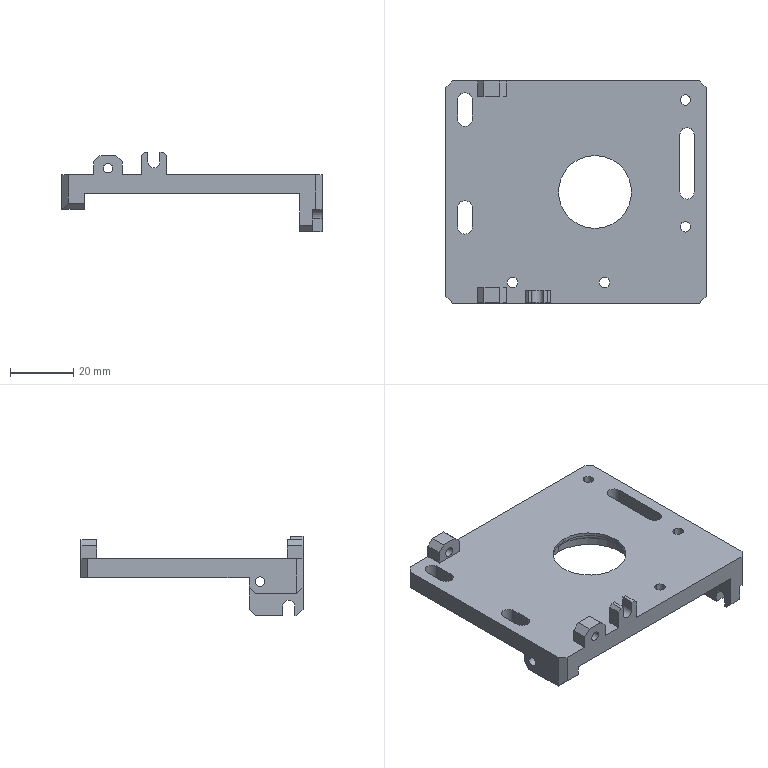NC program | NX | posted with a generic post | part box 82 x 70 x 25 mm
Lines 5584 to 7083 of 7981:
(CAVITY_MILL_COPY , TOOL : D4)
N11148 T04 M6
N11150 G54
N11152 G17 G0 G90 X-14.17 Y-28.2 S9500 M3
N11154 G43 Z30. H4
N11156 Z0.25
N11158 G94 G1 Z-0.25 F1800.
N11160 X-14.123 Y-28.364
N11162 G3 X-13.407 Y-29.062 R1.
N11164 G2 X-12. Y-30.376 R2.
N11166 X-10.593 Y-29.062 R2.
N11168 G3 X-9.877 Y-28.364 R1.
N11170 G1 X-9.83 Y-28.2
N11172 Z0.25
N11174 G0 Z30.
N11176 X-14.17
N11178 Z0.
N11180 G1 Z-0.5
N11182 X-14.123 Y-28.364
N11184 G3 X-13.407 Y-29.062 R1.
N11186 G2 X-12. Y-30.376 R2.
N11188 X-10.593 Y-29.062 R2.
N11190 G3 X-9.877 Y-28.364 R1.
N11192 G1 X-9.83 Y-28.2
N11194 Z0.
N11196 G0 X-14.17 Z-0.25
N11198 G1 Z-0.75
N11200 X-14.123 Y-28.364
N11202 G3 X-13.407 Y-29.062 R1.
N11204 G2 X-12. Y-30.376 R2.
N11206 X-10.593 Y-29.062 R2.
N11208 G3 X-9.877 Y-28.364 R1.
N11210 G1 X-9.83 Y-28.2
N11212 Z-0.25
N11214 G0 X-14.17 Z-0.5
N11216 G1 Z-1.
N11218 X-14.123 Y-28.364
N11220 G3 X-13.407 Y-29.062 R1.
N11222 G2 X-12. Y-30.376 R2.
N11224 X-10.593 Y-29.062 R2.
N11226 G3 X-9.877 Y-28.364 R1.
N11228 G1 X-9.83 Y-28.2
N11230 Z-0.5
N11232 G0 X-21.047 Y-28.181 Z-0.75
N11234 G1 Z-1.25
N11236 X-20.521 Y-29.33
N11238 G3 X-19.706 Y-29.909 R1.
N11240 G1 X-19.875 Y-31.701
N11242 X-19.95 Y-31.693
N11244 Y-33.841
N11246 X-19.8
N11248 Y-31.707
N11250 X-19.875 Y-31.701
N11252 X-19.706 Y-29.909
N11254 X-19.75 Y-29.904
N11256 G2 X-21.552 Y-28.819 R2.52
N11258 G3 X-22.241 Y-28.689 R0.5
N11260 G2 X-21.75 Y-30. R2.002
N11262 G1 Y-35.
N11264 G2 X-22.401 Y-36.474 R2.003
N11266 G3 X-21.712 Y-36.436 R0.5
N11268 G2 X-18.043 Y-36.43 R2.52
N11270 G3 X-17.357 Y-36.469 R0.5
N11272 G2 X-18. Y-35. R2.
N11274 G1 Y-31.
N11276 G2 X-17.172 Y-29.379 R2.
N11278 G3 X-17.857 Y-29.336 R0.5
N11280 G2 X-19.706 Y-29.909 R2.52
N11282 X-20.521 Y-29.33 R1.
N11284 G1 X-21.047 Y-28.181
N11286 Z-0.75
N11288 G0 X-18.039 Y-28.483 Z-1.
N11290 G1 Z-1.5
N11292 X-18.726 Y-29.376
N11294 G2 X-19.65 Y-29.758 R1.
N11296 X-21.319 Y-28.792 R2.52
N11298 G3 X-21.996 Y-28.681 R0.5
N11300 G2 X-21.5 Y-30. R2.
N11302 G1 Y-35.
N11304 G2 X-22.304 Y-36.603 R2.
N11306 G3 X-21.604 Y-36.623 R0.5
N11308 G1 X-21.45 Y-36.48
N11310 G2 X-17.979 Y-36.517 R2.52
N11312 G3 X-17.292 Y-36.527 R0.5
N11314 G2 X-18. Y-35. R2.
N11316 G1 Y-31.
N11318 G2 X-17.104 Y-29.332 R2.
N11320 G3 X-17.787 Y-29.261 R0.5
N11322 G2 X-19.65 Y-29.758 R2.52
N11324 X-20.443 Y-29.148 R1.
N11326 G1 X-20.873 Y-28.106
N11328 Z-1.
N11330 G0 X-17.936 Y-28.402 Z-1.25
N11332 G1 Z-1.75
N11334 X-18.678 Y-29.269
N11336 G2 X-19.621 Y-29.602 R1.
N11338 X-21.111 Y-28.719 R2.52
N11340 G3 X-21.792 Y-28.631 R0.5
N11342 G2 X-21.25 Y-30. R2.
N11344 G1 Y-35.
N11346 G2 X-22. Y-36.562 R2.
N11348 G3 X-21.317 Y-36.574 R0.5
N11350 G2 X-17.929 Y-36.579 R2.52
N11352 G3 X-17.243 Y-36.567 R0.5
N11354 G2 X-18. Y-35. R2.
N11356 G1 Y-31.
N11358 G2 X-17.034 Y-29.288 R2.
N11360 G3 X-17.713 Y-29.188 R0.5
N11362 G2 X-19.621 Y-29.602 R2.52
N11364 X-20.381 Y-28.952 R1.
N11366 G1 X-20.719 Y-27.995
N11368 Z-1.25
N11370 G0 X-17.828 Y-28.324 Z-1.5
N11372 G1 Z-2.
N11374 X-18.624 Y-29.161
N11376 G2 X-19.583 Y-29.445 R1.
N11378 X-20.906 Y-28.635 R2.52
N11380 G1 X-20.927 Y-28.611
N11382 G3 X-21.623 Y-28.55 R0.5
N11384 G2 X-21. Y-30. R2.
N11386 G1 Y-35.
N11388 G2 X-21.822 Y-36.616 R2.
N11390 G3 X-21.133 Y-36.654 R0.5
N11392 G2 X-17.871 Y-36.648 R2.52
N11394 G3 X-17.185 Y-36.611 R0.5
N11396 G2 X-18. Y-35. R2.
N11398 G1 Y-31.
N11400 G2 X-16.96 Y-29.246 R2.
N11402 G3 X-17.635 Y-29.118 R0.5
N11404 G2 X-19.583 Y-29.445 R2.52
N11406 X-20.308 Y-28.756 R1.
N11408 G1 X-20.571 Y-27.864
N11410 Z-1.5
N11412 G0 X-17.729 Y-28.258 Z-1.75
N11414 G1 Z-2.25
N11416 X-18.572 Y-29.066
N11418 G2 X-19.543 Y-29.304 R1.
N11420 X-20.691 Y-28.594 R2.52
N11422 G3 X-21.375 Y-28.547 R0.5
N11424 G2 X-20.75 Y-30. R2.
N11426 G1 Y-35.
N11428 G2 X-21.677 Y-36.688 R2.
N11430 G3 X-20.982 Y-36.762 R0.5
N11432 G1 X-20.928 Y-36.719
N11434 G2 X-17.81 Y-36.715 R2.52
N11436 G3 X-17.126 Y-36.653 R0.5
N11438 G2 X-18. Y-35. R2.
N11440 G1 Y-31.
N11442 G2 X-16.893 Y-29.211 R2.
N11444 G3 X-17.563 Y-29.057 R0.5
N11446 G2 X-19.543 Y-29.304 R2.52
N11448 X-20.235 Y-28.583 R1.
N11450 G1 X-20.428 Y-27.796
N11452 Z-1.75
N11454 G0 X-17.623 Y-28.193 Z-2.
N11456 G1 Z-2.5
N11458 X-18.512 Y-28.969
N11460 G2 X-19.494 Y-29.161 R1.
N11462 X-20.481 Y-28.537 R2.52
N11464 G3 X-21.167 Y-28.509 R0.5
N11466 G2 X-20.5 Y-30. R2.
N11468 G1 Y-35.
N11470 G2 X-21.439 Y-36.695 R2.
N11472 G3 X-20.753 Y-36.78 R0.5
N11474 G2 X-17.754 Y-36.772 R2.52
N11476 G3 X-17.073 Y-36.688 R0.5
N11478 G2 X-18. Y-35. R2.
N11480 G1 Y-31.
N11482 G2 X-16.823 Y-29.177 R2.
N11484 G3 X-17.486 Y-28.998 R0.5
N11486 G2 X-19.494 Y-29.161 R2.52
N11488 X-20.151 Y-28.408 R1.
N11490 G1 X-20.288 Y-27.709
N11492 Z-2.
N11494 G0 X-17.516 Y-28.133 Z-2.25
N11496 G1 Z-2.75
N11498 X-18.449 Y-28.874
N11500 G2 X-19.438 Y-29.021 R1.
N11502 X-20.274 Y-28.479 R2.52
N11504 G3 X-20.962 Y-28.47 R0.5
N11506 G2 X-20.25 Y-30. R2.
N11508 G1 Y-35.
N11510 G2 X-21.231 Y-36.721 R2.
N11512 G3 X-20.553 Y-36.827 R0.5
N11514 G2 X-17.697 Y-36.827 R2.52
N11516 G3 X-17.018 Y-36.721 R0.5
N11518 G2 X-18. Y-35. R2.
N11520 G1 Y-31.
N11522 G2 X-16.752 Y-29.147 R2.
N11524 G3 X-17.407 Y-28.942 R0.5
N11526 G2 X-19.438 Y-29.021 R2.52
N11528 X-20.06 Y-28.237 R1.
N11530 G1 X-20.151 Y-27.626
N11532 Z-2.25
N11534 G0 X-17.41 Y-28.079 Z-2.5
N11536 G1 Z-3.
N11538 X-18.383 Y-28.784
N11540 G2 X-19.378 Y-28.886 R1.
N11542 X-20.062 Y-28.434 R2.52
N11544 G3 X-20.75 Y-28.441 R0.5
N11546 G2 X-20. Y-30.007 R2.009
N11548 G1 Y-34.992
N11550 G2 X-21.039 Y-36.752 R2.004
N11552 G3 X-20.364 Y-36.879 R0.5
N11554 G2 X-17.639 Y-36.879 R2.52
N11556 G3 X-16.964 Y-36.752 R0.5
N11558 G2 X-18. Y-35. R2.
N11560 G1 Y-31.
N11562 G2 X-16.682 Y-29.12 R2.
N11564 G3 X-17.33 Y-28.891 R0.5
N11566 G2 X-19.378 Y-28.886 R2.52
N11568 X-19.964 Y-28.076 R1.
N11570 G1 X-20.018 Y-27.559
N11572 Z-2.5
N11574 G0 X-17.409 Y-28.079 Z-2.75
N11576 G1 Z-3.25
N11578 X-18.383 Y-28.783
N11580 G2 X-19.378 Y-28.885 R1.
N11582 X-20.059 Y-28.435 R2.52
N11584 G3 X-20.745 Y-28.443 R0.5
N11586 G2 X-20. Y-30. R2.
N11588 G1 Y-35.
N11590 G2 X-21.037 Y-36.753 R2.
N11592 G3 X-20.362 Y-36.88 R0.5
N11594 G2 X-17.638 Y-36.88 R2.52
N11596 G3 X-16.963 Y-36.753 R0.5
N11598 G2 X-18. Y-35. R2.
N11600 G1 Y-31.
N11602 G2 X-16.682 Y-29.12 R2.
N11604 G3 X-17.329 Y-28.89 R0.5
N11606 G2 X-19.378 Y-28.885 R2.52
N11608 X-19.964 Y-28.075 R1.
N11610 G1 X-20.017 Y-27.56
N11612 Z-2.75
N11614 G0 X-17.409 Y-28.079 Z-3.
N11616 G1 Z-3.5
N11618 X-18.383 Y-28.783
N11620 G2 X-19.378 Y-28.885 R1.
N11622 X-20.059 Y-28.435 R2.52
N11624 G3 X-20.745 Y-28.443 R0.5
N11626 G2 X-20. Y-30. R2.
N11628 G1 Y-35.
N11630 G2 X-21.037 Y-36.753 R2.
N11632 G3 X-20.362 Y-36.88 R0.5
N11634 G2 X-17.638 Y-36.88 R2.52
N11636 G3 X-16.963 Y-36.753 R0.5
N11638 G2 X-18. Y-35. R2.
N11640 G1 Y-31.
N11642 G2 X-16.682 Y-29.12 R2.
N11644 G3 X-17.329 Y-28.89 R0.5
N11646 G2 X-19.378 Y-28.885 R2.52
N11648 X-19.964 Y-28.075 R1.
N11650 G1 X-20.017 Y-27.56
N11652 Z-3.
N11654 G0 X-17.409 Y-28.079 Z-3.25
N11656 G1 Z-3.75
N11658 X-18.383 Y-28.783
N11660 G2 X-19.378 Y-28.885 R1.
N11662 X-20.059 Y-28.435 R2.52
N11664 G3 X-20.745 Y-28.443 R0.5
N11666 G2 X-20. Y-30. R2.
N11668 G1 Y-35.
N11670 G2 X-21.037 Y-36.753 R2.
N11672 G3 X-20.362 Y-36.88 R0.5
N11674 G2 X-17.638 Y-36.88 R2.52
N11676 G3 X-16.963 Y-36.753 R0.5
N11678 G2 X-18. Y-35. R2.
N11680 G1 Y-31.
N11682 G2 X-16.682 Y-29.12 R2.
N11684 G3 X-17.329 Y-28.89 R0.5
N11686 G2 X-19.378 Y-28.885 R2.52
N11688 X-19.964 Y-28.075 R1.
N11690 G1 X-20.017 Y-27.56
N11692 Z-3.25
N11694 G0 X-17.409 Y-28.079 Z-3.5
N11696 G1 Z-4.
N11698 X-18.383 Y-28.783
N11700 G2 X-19.378 Y-28.885 R1.
N11702 X-20.059 Y-28.435 R2.52
N11704 G3 X-20.745 Y-28.443 R0.5
N11706 G2 X-20. Y-30. R2.
N11708 G1 Y-35.
N11710 G2 X-21.037 Y-36.753 R2.
N11712 G3 X-20.362 Y-36.88 R0.5
N11714 G2 X-17.638 Y-36.88 R2.52
N11716 G3 X-16.963 Y-36.753 R0.5
N11718 G2 X-18. Y-35. R2.
N11720 G1 Y-31.
N11722 G2 X-16.682 Y-29.12 R2.
N11724 G3 X-17.329 Y-28.89 R0.5
N11726 G2 X-19.378 Y-28.885 R2.52
N11728 X-19.964 Y-28.075 R1.
N11730 G1 X-20.017 Y-27.56
N11732 Z-3.5
N11734 G0 X-17.409 Y-28.079 Z-3.75
N11736 G1 Z-4.25
N11738 X-18.383 Y-28.783
N11740 G2 X-19.378 Y-28.885 R1.
N11742 X-20.059 Y-28.435 R2.52
N11744 G3 X-20.745 Y-28.443 R0.5
N11746 G2 X-20. Y-30. R2.
N11748 G1 Y-35.
N11750 G2 X-21.037 Y-36.753 R2.
N11752 G3 X-20.362 Y-36.88 R0.5
N11754 G2 X-17.638 Y-36.88 R2.52
N11756 G3 X-16.963 Y-36.753 R0.5
N11758 G2 X-18. Y-35. R2.
N11760 G1 Y-31.
N11762 G2 X-16.682 Y-29.12 R2.
N11764 G3 X-17.329 Y-28.89 R0.5
N11766 G2 X-19.378 Y-28.885 R2.52
N11768 X-19.964 Y-28.075 R1.
N11770 G1 X-20.017 Y-27.56
N11772 Z-3.75
N11774 G0 X-17.409 Y-28.079 Z-4.
N11776 G1 Z-4.5
N11778 X-18.383 Y-28.783
N11780 G2 X-19.378 Y-28.885 R1.
N11782 X-20.059 Y-28.435 R2.52
N11784 G3 X-20.745 Y-28.443 R0.5
N11786 G2 X-20. Y-30. R2.
N11788 G1 Y-35.
N11790 G2 X-21.037 Y-36.753 R2.
N11792 G3 X-20.362 Y-36.88 R0.5
N11794 G2 X-17.638 Y-36.88 R2.52
N11796 G3 X-16.963 Y-36.753 R0.5
N11798 G2 X-18. Y-35. R2.
N11800 G1 Y-31.
N11802 G2 X-16.682 Y-29.12 R2.
N11804 G3 X-17.329 Y-28.89 R0.5
N11806 G2 X-19.378 Y-28.885 R2.52
N11808 X-19.964 Y-28.075 R1.
N11810 G1 X-20.017 Y-27.56
N11812 Z-4.
N11814 G0 X-17.409 Y-28.079 Z-4.25
N11816 G1 Z-4.75
N11818 X-18.383 Y-28.783
N11820 G2 X-19.378 Y-28.885 R1.
N11822 X-20.059 Y-28.435 R2.52
N11824 G3 X-20.745 Y-28.443 R0.5
N11826 G2 X-20. Y-30. R2.
N11828 G1 Y-35.
N11830 G2 X-21.037 Y-36.753 R2.
N11832 G3 X-20.362 Y-36.88 R0.5
N11834 G2 X-17.638 Y-36.88 R2.52
N11836 G3 X-16.963 Y-36.753 R0.5
N11838 G2 X-18. Y-35. R2.
N11840 G1 Y-31.
N11842 G2 X-16.682 Y-29.12 R2.
N11844 G3 X-17.329 Y-28.89 R0.5
N11846 G2 X-19.378 Y-28.885 R2.52
N11848 X-19.964 Y-28.075 R1.
N11850 G1 X-20.017 Y-27.56
N11852 Z-4.25
N11854 G0 X-17.409 Y-28.079 Z-4.5
N11856 G1 Z-5.
N11858 X-18.383 Y-28.783
N11860 G2 X-19.378 Y-28.885 R1.
N11862 X-20.059 Y-28.435 R2.52
N11864 G3 X-20.745 Y-28.443 R0.5
N11866 G2 X-20. Y-30. R2.
N11868 G1 Y-35.
N11870 G2 X-21.037 Y-36.753 R2.
N11872 G3 X-20.362 Y-36.88 R0.5
N11874 G2 X-17.638 Y-36.88 R2.52
N11876 G3 X-16.963 Y-36.753 R0.5
N11878 G2 X-18. Y-35. R2.
N11880 G1 Y-31.
N11882 G2 X-16.682 Y-29.12 R2.
N11884 G3 X-17.329 Y-28.89 R0.5
N11886 G2 X-19.378 Y-28.885 R2.52
N11888 X-19.964 Y-28.075 R1.
N11890 G1 X-20.017 Y-27.56
N11892 Z-4.5
N11894 G0 X-17.409 Y-28.079 Z-4.75
N11896 G1 Z-5.25
N11898 X-18.383 Y-28.783
N11900 G2 X-19.378 Y-28.885 R1.
N11902 X-20.059 Y-28.435 R2.52
N11904 G3 X-20.745 Y-28.443 R0.5
N11906 G2 X-20. Y-30. R2.
N11908 G1 Y-35.
N11910 G2 X-21.037 Y-36.753 R2.
N11912 G3 X-20.362 Y-36.88 R0.5
N11914 G2 X-17.638 Y-36.88 R2.52
N11916 G3 X-16.963 Y-36.753 R0.5
N11918 G2 X-18. Y-35. R2.
N11920 G1 Y-31.
N11922 G2 X-16.682 Y-29.12 R2.
N11924 G3 X-17.329 Y-28.89 R0.5
N11926 G2 X-19.378 Y-28.885 R2.52
N11928 X-19.964 Y-28.075 R1.
N11930 G1 X-20.017 Y-27.56
N11932 Z-4.75
N11934 G0 X-17.409 Y-28.079 Z-5.
N11936 G1 Z-5.5
N11938 X-18.383 Y-28.783
N11940 G2 X-19.378 Y-28.885 R1.
N11942 X-20.059 Y-28.435 R2.52
N11944 G3 X-20.745 Y-28.443 R0.5
N11946 G2 X-20. Y-30. R2.
N11948 G1 Y-35.
N11950 G2 X-21.037 Y-36.753 R2.
N11952 G3 X-20.362 Y-36.88 R0.5
N11954 G2 X-17.638 Y-36.88 R2.52
N11956 G3 X-16.963 Y-36.753 R0.5
N11958 G2 X-18. Y-35. R2.
N11960 G1 Y-31.
N11962 G2 X-16.682 Y-29.12 R2.
N11964 G3 X-17.329 Y-28.89 R0.5
N11966 G2 X-19.378 Y-28.885 R2.52
N11968 X-19.964 Y-28.075 R1.
N11970 G1 X-20.017 Y-27.56
N11972 Z-5.
N11974 G0 X-17.409 Y-28.079 Z-5.25
N11976 G1 Z-5.75
N11978 X-18.383 Y-28.783
N11980 G2 X-19.378 Y-28.885 R1.
N11982 X-20.059 Y-28.435 R2.52
N11984 G3 X-20.745 Y-28.443 R0.5
N11986 G2 X-20. Y-30. R2.
N11988 G1 Y-35.
N11990 G2 X-21.037 Y-36.753 R2.
N11992 G3 X-20.362 Y-36.88 R0.5
N11994 G2 X-17.638 Y-36.88 R2.52
N11996 G3 X-16.963 Y-36.753 R0.5
N11998 G2 X-18. Y-35. R2.
N12000 G1 Y-31.
N12002 G2 X-16.682 Y-29.12 R2.
N12004 G3 X-17.329 Y-28.89 R0.5
N12006 G2 X-19.378 Y-28.885 R2.52
N12008 X-19.964 Y-28.075 R1.
N12010 G1 X-20.017 Y-27.56
N12012 Z-5.25
N12014 G0 X-17.409 Y-28.079 Z-5.5
N12016 G1 Z-6.
N12018 X-18.383 Y-28.783
N12020 G2 X-19.378 Y-28.885 R1.
N12022 X-20.059 Y-28.435 R2.52
N12024 G3 X-20.745 Y-28.443 R0.5
N12026 G2 X-20. Y-30. R2.
N12028 G1 Y-35.
N12030 G2 X-21.037 Y-36.753 R2.
N12032 G3 X-20.362 Y-36.88 R0.5
N12034 G2 X-17.638 Y-36.88 R2.52
N12036 G3 X-16.963 Y-36.753 R0.5
N12038 G2 X-18. Y-35. R2.
N12040 G1 Y-31.
N12042 G2 X-16.682 Y-29.12 R2.
N12044 G3 X-17.329 Y-28.89 R0.5
N12046 G2 X-19.378 Y-28.885 R2.52
N12048 X-19.964 Y-28.075 R1.
N12050 G1 X-20.017 Y-27.56
N12052 Z-5.5
N12054 G0 X-17.409 Y-28.079 Z-5.75
N12056 G1 Z-6.25
N12058 X-18.383 Y-28.783
N12060 G2 X-19.378 Y-28.885 R1.
N12062 X-20.059 Y-28.435 R2.52
N12064 G3 X-20.745 Y-28.443 R0.5
N12066 G2 X-20. Y-30. R2.
N12068 G1 Y-35.
N12070 G2 X-21.037 Y-36.753 R2.
N12072 G3 X-20.362 Y-36.88 R0.5
N12074 G2 X-17.638 Y-36.88 R2.52
N12076 G3 X-16.963 Y-36.753 R0.5
N12078 G2 X-18. Y-35. R2.
N12080 G1 Y-31.
N12082 G2 X-16.682 Y-29.12 R2.
N12084 G3 X-17.329 Y-28.89 R0.5
N12086 G2 X-19.378 Y-28.885 R2.52
N12088 X-19.964 Y-28.075 R1.
N12090 G1 X-20.017 Y-27.56
N12092 Z-5.75
N12094 G0 X-17.409 Y-28.079 Z-6.
N12096 G1 Z-6.5
N12098 X-18.383 Y-28.783
N12100 G2 X-19.378 Y-28.885 R1.
N12102 X-20.059 Y-28.435 R2.52
N12104 G3 X-20.745 Y-28.443 R0.5
N12106 G2 X-20. Y-30. R2.
N12108 G1 Y-35.
N12110 G2 X-21.037 Y-36.753 R2.
N12112 G3 X-20.362 Y-36.88 R0.5
N12114 G2 X-17.638 Y-36.88 R2.52
N12116 G3 X-16.963 Y-36.753 R0.5
N12118 G2 X-18. Y-35. R2.
N12120 G1 Y-31.
N12122 G2 X-16.682 Y-29.12 R2.
N12124 G3 X-17.329 Y-28.89 R0.5
N12126 G2 X-19.378 Y-28.885 R2.52
N12128 X-19.964 Y-28.075 R1.
N12130 G1 X-20.017 Y-27.56
N12132 Z-6.
N12134 G0 X-17.409 Y-28.079 Z-6.25
N12136 G1 Z-6.75
N12138 X-18.383 Y-28.783
N12140 G2 X-19.378 Y-28.885 R1.
N12142 X-20.059 Y-28.435 R2.52
N12144 G3 X-20.745 Y-28.443 R0.5
N12146 G2 X-20. Y-30. R2.
N12148 G1 Y-35.
N12150 G2 X-21.037 Y-36.753 R2.
N12152 G3 X-20.362 Y-36.88 R0.5
N12154 G2 X-17.638 Y-36.88 R2.52
N12156 G3 X-16.963 Y-36.753 R0.5
N12158 G2 X-18. Y-35. R2.
N12160 G1 Y-31.
N12162 G2 X-16.682 Y-29.12 R2.
N12164 G3 X-17.329 Y-28.89 R0.5
N12166 G2 X-19.378 Y-28.885 R2.52
N12168 X-19.964 Y-28.075 R1.
N12170 G1 X-20.017 Y-27.56
N12172 Z-6.25
N12174 G0 X-17.409 Y-28.079 Z-6.5
N12176 G1 Z-7.
N12178 X-18.383 Y-28.783
N12180 G2 X-19.378 Y-28.885 R1.
N12182 X-20.059 Y-28.435 R2.52
N12184 G3 X-20.745 Y-28.443 R0.5
N12186 G2 X-20. Y-30. R2.
N12188 G1 Y-35.
N12190 G2 X-21.037 Y-36.753 R2.
N12192 G3 X-20.362 Y-36.88 R0.5
N12194 G2 X-17.638 Y-36.88 R2.52
N12196 G3 X-16.963 Y-36.753 R0.5
N12198 G2 X-18. Y-35. R2.
N12200 G1 Y-31.
N12202 G2 X-16.682 Y-29.12 R2.
N12204 G3 X-17.329 Y-28.89 R0.5
N12206 G2 X-19.378 Y-28.885 R2.52
N12208 X-19.964 Y-28.075 R1.
N12210 G1 X-20.017 Y-27.56
N12212 Z-6.5
N12214 G0 Z9.
N12216 X-14.17 Y-28.2
N12218 Z-0.75
N12220 G1 Z-1.25
N12222 X-14.123 Y-28.364
N12224 G3 X-13.407 Y-29.062 R1.
N12226 G2 X-12. Y-30.376 R2.
N12228 X-10.593 Y-29.062 R2.
N12230 G3 X-9.877 Y-28.364 R1.
N12232 G1 X-9.83 Y-28.2
N12234 Z-0.75
N12236 G0 X-14.17 Z-1.
N12238 G1 Z-1.5
N12240 X-14.123 Y-28.364
N12242 G3 X-13.407 Y-29.062 R1.
N12244 G2 X-12. Y-30.376 R2.
N12246 X-10.593 Y-29.062 R2.
N12248 G3 X-9.877 Y-28.364 R1.
N12250 G1 X-9.83 Y-28.2
N12252 Z-1.
N12254 G0 X-14.17 Z-1.25
N12256 G1 Z-1.75
N12258 X-14.123 Y-28.364
N12260 G3 X-13.407 Y-29.062 R1.
N12262 G2 X-12. Y-30.376 R2.
N12264 X-10.593 Y-29.062 R2.
N12266 G3 X-9.877 Y-28.364 R1.
N12268 G1 X-9.83 Y-28.2
N12270 Z-1.25
N12272 G0 X-14.17 Z-1.5
N12274 G1 Z-2.
N12276 X-14.123 Y-28.364
N12278 G3 X-13.407 Y-29.062 R1.
N12280 G2 X-12. Y-30.376 R2.
N12282 X-10.593 Y-29.062 R2.
N12284 G3 X-9.877 Y-28.364 R1.
N12286 G1 X-9.83 Y-28.2
N12288 Z-1.5
N12290 G0 X-14.17 Z-1.75
N12292 G1 Z-2.25
N12294 X-14.123 Y-28.364
N12296 G3 X-13.407 Y-29.062 R1.
N12298 G2 X-12. Y-30.376 R2.
N12300 X-10.593 Y-29.062 R2.
N12302 G3 X-9.877 Y-28.364 R1.
N12304 G1 X-9.83 Y-28.2
N12306 Z-1.75
N12308 G0 X-14.17 Z-2.
N12310 G1 Z-2.5
N12312 X-14.123 Y-28.364
N12314 G3 X-13.407 Y-29.062 R1.
N12316 G2 X-12. Y-30.376 R2.
N12318 X-10.593 Y-29.062 R2.
N12320 G3 X-9.877 Y-28.364 R1.
N12322 G1 X-9.83 Y-28.2
N12324 Z-2.
N12326 G0 X-14.17 Z-2.25
N12328 G1 Z-2.75
N12330 X-14.123 Y-28.364
N12332 G3 X-13.407 Y-29.062 R1.
N12334 G2 X-12. Y-30.376 R2.
N12336 X-10.593 Y-29.062 R2.
N12338 G3 X-9.877 Y-28.364 R1.
N12340 G1 X-9.83 Y-28.2
N12342 Z-2.25
N12344 G0 X-14.17 Z-2.5
N12346 G1 Z-3.
N12348 X-14.123 Y-28.364
N12350 G3 X-13.407 Y-29.062 R1.
N12352 G2 X-12. Y-30.376 R2.
N12354 X-10.593 Y-29.062 R2.
N12356 G3 X-9.877 Y-28.364 R1.
N12358 G1 X-9.83 Y-28.2
N12360 Z-2.5
N12362 G0 X-14.183 Z-2.75
N12364 G1 Z-3.25
N12366 X-14.134 Y-28.367
N12368 G3 X-13.408 Y-29.055 R1.
N12370 G2 X-12.035 Y-30.222 R1.993
N12372 G1 X-11.997 Y-30.314
N12374 G2 X-10.609 Y-29.057 R1.975
N12376 G3 X-9.888 Y-28.364 R1.
N12378 G1 X-9.841 Y-28.2
N12380 Z-2.75
N12382 G0 X-14.173 Z-3.
N12384 G1 Z-3.5
N12386 X-14.12 Y-28.37
N12388 G3 X-13.385 Y-29.048 R1.
N12390 G2 X-12. Y-30.18 R1.998
N12392 X-10.611 Y-29.047 R1.998
N12394 G3 X-9.874 Y-28.371 R1.
N12396 G1 X-9.821 Y-28.2
N12398 Z-3.
N12400 G0 X-14.129 Z-3.25
N12402 G1 Z-3.75
N12404 X-14.072 Y-28.375
N12406 G3 X-13.328 Y-29.043 R1.
N12408 G2 X-12.003 Y-30.008 R2.002
N12410 G1 X-11.751 Y-29.657
N12412 G2 X-11.138 Y-29.195 R2.638
N12414 X-10.715 Y-29.052 R2.143
N12416 G3 X-9.98 Y-28.374 R1.
N12418 G1 X-9.925 Y-28.2
N12420 Z-3.25
N12422 G0 X-14.089 Z-3.5
N12424 G1 Z-4.
N12426 X-14.021 Y-28.387
N12428 G3 X-13.256 Y-29.031 R1.
N12430 G2 X-11.996 Y-29.805 R2.02
N12432 X-10.771 Y-29.035 R1.986
N12434 G3 X-10.015 Y-28.382 R1.
N12436 G1 X-9.951 Y-28.2
N12438 Z-3.5
N12440 G0 X-13.99 Z-3.75
N12442 G1 Z-4.25
N12444 X-13.911 Y-28.4
N12446 G3 X-13.127 Y-29.021 R1.
N12448 G2 X-12.002 Y-29.593 R1.981
N12450 X-10.873 Y-29.022 R2.002
N12452 G3 X-10.089 Y-28.4 R1.
N12454 G1 X-10.01 Y-28.2
N12456 Z-3.75
N12458 G0 X-13.902 Z-4.
N12460 G1 Z-4.5
N12462 X-13.794 Y-28.432
N12464 G3 X-12.976 Y-29.008 R1.
N12466 G2 X-12.002 Y-29.364 R2.016
N12468 X-10.998 Y-29.006 R2.041
N12470 G3 X-10.174 Y-28.44 R1.
N12472 G1 X-10.059 Y-28.2
N12474 Z-4.
N12476 G0 X-13.813 Z-4.25
N12478 G1 Z-4.75
N12480 X-13.64 Y-28.5
N12482 G3 X-12.774 Y-29. R1.
N12484 G1 X-12.737
N12486 G2 X-12.002 Y-29.133 R2.498
N12488 X-11.267 Y-29. R2.58
N12490 G3 X-10.418 Y-28.472 R1.
N12492 G1 X-10.273 Y-28.2
N12494 Z-4.25
N12496 G0 Z30.
N12498 X-9.83 Y-37.8
N12500 Z0.25
N12502 G1 Z-0.25
N12504 X-9.877 Y-37.636
N12506 G3 X-10.593 Y-36.938 R1.
N12508 G2 X-12. Y-35.625 R2.
N12510 X-13.407 Y-36.938 R2.
N12512 G3 X-14.123 Y-37.636 R1.
N12514 G1 X-14.17 Y-37.8
N12516 Z0.25
N12518 G0 Z30.
N12520 X-9.83
N12522 Z0.
N12524 G1 Z-0.5
N12526 X-9.877 Y-37.636
N12528 G3 X-10.593 Y-36.938 R1.
N12530 G2 X-12. Y-35.625 R2.
N12532 X-13.407 Y-36.938 R2.
N12534 G3 X-14.123 Y-37.636 R1.
N12536 G1 X-14.17 Y-37.8
N12538 Z0.
N12540 G0 X-9.83 Z-0.25
N12542 G1 Z-0.75
N12544 X-9.877 Y-37.636
N12546 G3 X-10.593 Y-36.938 R1.
N12548 G2 X-12. Y-35.625 R2.
N12550 X-13.407 Y-36.938 R2.
N12552 G3 X-14.123 Y-37.636 R1.
N12554 G1 X-14.17 Y-37.8
N12556 Z-0.25
N12558 G0 X-9.83 Z-0.5
N12560 G1 Z-1.
N12562 X-9.877 Y-37.636
N12564 G3 X-10.593 Y-36.938 R1.
N12566 G2 X-12. Y-35.625 R2.
N12568 X-13.407 Y-36.938 R2.
N12570 G3 X-14.123 Y-37.636 R1.
N12572 G1 X-14.17 Y-37.8
N12574 Z-0.5
N12576 G0 X-9.83 Z-0.75
N12578 G1 Z-1.25
N12580 X-9.877 Y-37.636
N12582 G3 X-10.593 Y-36.938 R1.
N12584 G2 X-12. Y-35.625 R2.
N12586 X-13.407 Y-36.938 R2.
N12588 G3 X-14.123 Y-37.636 R1.
N12590 G1 X-14.17 Y-37.8
N12592 Z-0.75
N12594 G0 X-9.83 Z-1.
N12596 G1 Z-1.5
N12598 X-9.877 Y-37.636
N12600 G3 X-10.593 Y-36.938 R1.
N12602 G2 X-12. Y-35.625 R2.
N12604 X-13.407 Y-36.938 R2.
N12606 G3 X-14.123 Y-37.636 R1.
N12608 G1 X-14.17 Y-37.8
N12610 Z-1.
N12612 G0 X-9.83 Z-1.25
N12614 G1 Z-1.75
N12616 X-9.877 Y-37.636
N12618 G3 X-10.593 Y-36.938 R1.
N12620 G2 X-12. Y-35.625 R2.
N12622 X-13.407 Y-36.938 R2.
N12624 G3 X-14.123 Y-37.636 R1.
N12626 G1 X-14.17 Y-37.8
N12628 Z-1.25
N12630 G0 X-9.83 Z-1.5
N12632 G1 Z-2.
N12634 X-9.877 Y-37.636
N12636 G3 X-10.593 Y-36.938 R1.
N12638 G2 X-12. Y-35.625 R2.
N12640 X-13.407 Y-36.938 R2.
N12642 G3 X-14.123 Y-37.636 R1.
N12644 G1 X-14.17 Y-37.8
N12646 Z-1.5
N12648 G0 X-9.83 Z-1.75
N12650 G1 Z-2.25
N12652 X-9.877 Y-37.636
N12654 G3 X-10.593 Y-36.938 R1.
N12656 G2 X-12. Y-35.625 R2.
N12658 X-13.407 Y-36.938 R2.
N12660 G3 X-14.123 Y-37.636 R1.
N12662 G1 X-14.17 Y-37.8
N12664 Z-1.75
N12666 G0 X-9.83 Z-2.
N12668 G1 Z-2.5
N12670 X-9.877 Y-37.636
N12672 G3 X-10.593 Y-36.938 R1.
N12674 G2 X-12. Y-35.625 R2.
N12676 X-13.407 Y-36.938 R2.
N12678 G3 X-14.123 Y-37.636 R1.
N12680 G1 X-14.17 Y-37.8
N12682 Z-2.
N12684 G0 X-9.83 Z-2.25
N12686 G1 Z-2.75
N12688 X-9.877 Y-37.636
N12690 G3 X-10.593 Y-36.938 R1.
N12692 G2 X-12. Y-35.625 R2.
N12694 X-13.407 Y-36.938 R2.
N12696 G3 X-14.123 Y-37.636 R1.
N12698 G1 X-14.17 Y-37.8
N12700 Z-2.25
N12702 G0 X-9.83 Z-2.5
N12704 G1 Z-3.
N12706 X-9.877 Y-37.636
N12708 G3 X-10.593 Y-36.938 R1.
N12710 G2 X-12. Y-35.625 R2.
N12712 X-13.407 Y-36.938 R2.
N12714 G3 X-14.123 Y-37.636 R1.
N12716 G1 X-14.17 Y-37.8
N12718 Z-2.5
N12720 G0 X-9.82 Z-2.75
N12722 G1 Z-3.25
N12724 X-9.869 Y-37.634
N12726 G3 X-10.594 Y-36.945 R1.
N12728 G2 X-11.997 Y-35.687 R1.981
N12730 X-12.548 Y-36.502 R2.278
N12732 X-13.41 Y-36.94 R2.001
N12734 G3 X-14.141 Y-37.622 R1.
N12736 G1 X-14.196 Y-37.8
N12738 Z-2.75
N12740 G0 X-9.838 Z-3.
N12742 G1 Z-3.5
N12744 X-9.89 Y-37.632
N12746 G3 X-10.622 Y-36.951 R1.
N12748 G2 X-11.998 Y-35.823 R1.996
N12750 X-13.37 Y-36.949 R2.009
N12752 G3 X-14.099 Y-37.633 R1.
N12754 G1 X-14.15 Y-37.8
N12756 Z-3.
N12758 G0 X-9.89 Z-3.25
N12760 G1 Z-3.75
N12762 X-9.946 Y-37.627
N12764 G3 X-10.686 Y-36.956 R1.
N12766 G2 X-11.702 Y-36.382 R1.968
N12768 X-11.998 Y-35.992 R1.309
N12770 X-13.312 Y-36.954 R2.009
N12772 G3 X-14.051 Y-37.627 R1.
N12774 G1 X-14.107 Y-37.8
N12776 Z-3.25
N12778 G0 X-9.921 Z-3.5
N12780 G1 Z-4.
N12782 X-9.987 Y-37.614
N12784 G3 X-10.75 Y-36.968 R1.
N12786 G2 X-11.998 Y-36.195 R2.003
N12788 X-13.24 Y-36.966 R2.018
N12790 G3 X-14. Y-37.616 R1.
N12792 G1 X-14.065 Y-37.8
N12794 Z-3.5
N12796 G0 X-9.999 Z-3.75
N12798 G1 Z-4.25
N12800 X-10.08 Y-37.599
N12802 G3 X-10.865 Y-36.979 R1.
N12804 G2 X-11.998 Y-36.409 R2.007
N12806 X-13.134 Y-36.978 R2.026
N12808 G3 X-13.918 Y-37.599 R1.
N12810 G1 X-13.998 Y-37.8
N12812 Z-3.75
N12814 G0 X-10.087 Z-4.
N12816 G1 Z-4.5
N12818 X-10.195 Y-37.566
N12820 G3 X-11.014 Y-36.992 R1.
N12822 G2 X-11.998 Y-36.632 R2.015
N12824 X-12.997 Y-36.993 R2.034
N12826 G3 X-13.819 Y-37.563 R1.
N12828 G1 X-13.931 Y-37.8
N12830 Z-4.
N12832 G0 X-10.22 Z-4.25
N12834 G1 Z-4.75
N12836 X-10.391 Y-37.502
N12838 G3 X-11.256 Y-37. R1.
N12840 G1 X-11.263
N12842 G2 X-11.984 Y-36.866 R2.075
N12844 X-12.752 Y-37. R2.475
N12846 G3 X-13.618 Y-37.5 R1.
N12848 G1 X-13.792 Y-37.8
N12850 Z-4.25
N12852 G0 Z30.
(FLOOR_WALL_1 , TOOL : D4)
N12854 X-32. Y34.999
N12856 Z-0.5
N12858 G1 Z-1. F1350.
N12860 X-31.
N12862 X-22.
N12864 Y33.3
N12866 X-31.
N12868 Y31.6
N12870 X-22.
N12872 X-21.
N12874 Z-0.5
N12876 G0 Z30.
N12878 X-43.244 Y34.999
N12880 Z-6.5
N12882 G1 Z-7.
N12884 X-41.829
N12886 X-33.2
N12888 Y33.045
N12890 X-43.
N12892 Y31.09
N12894 X-33.2
N12896 Y29.136
N12898 X-43.
N12900 X-44.
N12902 Z-6.5
N12904 G0 Z30.
N12906 X-22.039 Y38.
N12908 Z-6.4
N12910 G1 X-19.8 Z-7.
N12912 Y34.999
N12914 X41.829
N12916 X43. Y33.828
N12918 Y33.045
N12920 X-19.8
N12922 Y31.09
N12924 X43.
N12926 Y29.136
N12928 X-19.8
N12930 Z-6.5
N12932 G0 Z30.
N12934 X-44. Y27.182
N12936 Z-6.5
N12938 G1 Z-7.
N12940 X-43.
N12942 X43.
N12944 Y25.228
N12946 X-43.
N12948 Y23.273
N12950 X43.
N12952 Y21.319
N12954 X-43.
N12956 Y19.365
N12958 X43.
N12960 Y17.411
N12962 X-43.
N12964 Y15.456
N12966 X43.
N12968 Y13.502
N12970 X-43.
N12972 Y11.548
N12974 X43.
N12976 Y9.594
N12978 X-43.
N12980 Y7.639
N12982 X43.
N12984 Y5.685
N12986 X-43.
N12988 Y3.731
N12990 X43.
N12992 Y1.777
N12994 X-43.
N12996 Y-0.178
N12998 X43.
N13000 Y-2.132
N13002 X-43.
N13004 Y-4.086
N13006 X43.
N13008 Y-6.04
N13010 X-43.
N13012 Y-7.995
N13014 X43.
N13016 Y-9.949
N13018 X-43.
N13020 Y-11.903
N13022 X43.
N13024 Y-13.857
N13026 X-43.
N13028 Y-15.812
N13030 X43.
N13032 Y-17.766
N13034 X-43.
N13036 Y-19.72
N13038 X43.
N13040 Y-21.674
N13042 X-43.
N13044 Y-23.629
N13046 X43.
N13048 Y-25.583
N13050 X-43.
N13052 Y-27.537
N13054 X43.
N13056 Y-29.491
N13058 X-5.8
N13060 Y-31.446
N13062 X43.
N13064 Y-33.4
N13066 X-5.8
N13068 Y-35.354
N13070 X41.474
N13072 X42.888
N13074 Z-6.5
N13076 G0 Z30.
N13078 X-35.439 Y-37.
N13080 Z-6.4
N13082 G1 X-33.2 Z-7.
N13084 Y-29.491
N13086 X-43.
N13088 Y-31.446
N13090 X-33.2
N13092 Y-33.4
N13094 X-43.
N13096 Y-33.828
N13098 X-41.474 Y-35.354
N13100 X-33.2
N13102 Y-38.
N13104 Z-6.5
N13106 G0 Z30.
N13108 X-19.161 Y-37.
N13110 Z-6.4
N13112 G1 X-19.8 Z-6.571
N13114 X-18.2 Z-7.
N13116 Y-29.491
N13118 X-19.8
N13120 Y-31.446
N13122 X-18.2
N13124 Y-33.4
N13126 X-19.8
N13128 Y-35.354
N13130 X-18.2
N13132 Y-38.
N13134 Z-6.5
N13136 G0 Z30.
N13138 X-18.
N13140 Z-6.5
N13142 G1 Z-7.
N13144 Y-37.
N13146 Y-29.
N13148 X-6.
N13150 Y-37.
N13152 Y-38.
N13154 Z-6.5
N13156 G0 Z30.
N13158 X-20. Y38.
N13160 Z-6.5
N13162 G1 Z-7.
N13164 Y37.
N13166 Y28.
N13168 X-33.
N13170 Y37.
N13172 Y38.
N13174 Z-6.5
N13176 G0 Z30.
N13178 Y-38.
N13180 Z-6.5
N13182 G1 Z-7.
N13184 Y-37.
N13186 Y-28.
N13188 X-20.
N13190 Y-37.
N13192 Y-38.
N13194 Z-6.5
N13196 G0 Z30.
N13198 X-32. Y-30.001
N13200 Z-0.5
N13202 G1 Z-1.
N13204 X-31.
N13206 X-22.
N13208 Y-31.701
N13210 X-31.
N13212 Y-33.4
N13214 X-22.
N13216 X-21.
N13218 Z-0.5
N13220 G0 Z30.
N13222 M5
(CAVITY_MILL_COPY_COPY , TOOL : D3)
N13224 T03 M6
N13226 G54
N13228 G17 G0 G90 X-12.379 Y-36.448 S9500 M3
N13230 G43 Z30. H3
N13232 Z0.25
N13234 G94 G1 Z-0.25 F1800.
N13236 X-12.685 Y-36.043
N13238 G2 X-11.709 Y-35.826 R1.
N13240 G3 X-11.363 Y-35.809 R0.5
N13242 G2 X-11.6 Y-35. R1.5
N13244 G1 Y-31.
N13246 G2 X-11.363 Y-30.191 R1.5
N13248 G3 X-11.983 Y-30.386 R0.5
N13250 G1 X-11.99 Y-30.404
N13252 X-12.01
N13254 X-12.017 Y-30.386
N13256 G3 X-12.637 Y-30.191 R0.5
N13258 G2 X-12.4 Y-31. R1.5
N13260 G1 Y-35.
N13262 G2 X-12.637 Y-35.809 R1.5
N13264 G3 X-12.017 Y-35.614 R0.5
N13266 G1 X-12.01 Y-35.596
N13268 X-11.99
N13270 X-11.983 Y-35.614
N13272 G3 X-11.709 Y-35.826 R0.5
N13274 G2 X-11.033 Y-36.563 R1.
N13276 G1 X-10.955 Y-36.918
N13278 Z0.25
N13280 G0 Z30.
N13282 X-12.379 Y-36.448
N13284 Z0.
N13286 G1 Z-0.5
N13288 X-12.685 Y-36.043
N13290 G2 X-11.709 Y-35.826 R1.
N13292 G3 X-11.363 Y-35.809 R0.5
N13294 G2 X-11.6 Y-35. R1.5
N13296 G1 Y-31.
N13298 G2 X-11.363 Y-30.191 R1.5
N13300 G3 X-11.983 Y-30.386 R0.5
N13302 G1 X-11.99 Y-30.404
N13304 X-12.01
N13306 X-12.017 Y-30.386
N13308 G3 X-12.637 Y-30.191 R0.5
N13310 G2 X-12.4 Y-31. R1.5
N13312 G1 Y-35.
N13314 G2 X-12.637 Y-35.809 R1.5
N13316 G3 X-12.017 Y-35.614 R0.5
N13318 G1 X-12.01 Y-35.596
N13320 X-11.99
N13322 X-11.983 Y-35.614
N13324 G3 X-11.709 Y-35.826 R0.5
N13326 G2 X-11.033 Y-36.563 R1.
N13328 G1 X-10.955 Y-36.918
N13330 Z0.
N13332 G0 X-12.379 Y-36.448 Z-0.25
N13334 G1 Z-0.75
N13336 X-12.685 Y-36.043
N13338 G2 X-11.709 Y-35.826 R1.
N13340 G3 X-11.363 Y-35.809 R0.5
N13342 G2 X-11.6 Y-35. R1.5
N13344 G1 Y-31.
N13346 G2 X-11.363 Y-30.191 R1.5
N13348 G3 X-11.983 Y-30.386 R0.5
N13350 G1 X-11.99 Y-30.404
N13352 X-12.01
N13354 X-12.017 Y-30.386
N13356 G3 X-12.637 Y-30.191 R0.5
N13358 G2 X-12.4 Y-31. R1.5
N13360 G1 Y-35.
N13362 G2 X-12.637 Y-35.809 R1.5
N13364 G3 X-12.017 Y-35.614 R0.5
N13366 G1 X-12.01 Y-35.596
N13368 X-11.99
N13370 X-11.983 Y-35.614
N13372 G3 X-11.709 Y-35.826 R0.5
N13374 G2 X-11.033 Y-36.563 R1.
N13376 G1 X-10.955 Y-36.918
N13378 Z-0.25
N13380 G0 X-12.379 Y-36.448 Z-0.5
N13382 G1 Z-1.
N13384 X-12.685 Y-36.043
N13386 G2 X-11.709 Y-35.826 R1.
N13388 G3 X-11.363 Y-35.809 R0.5
N13390 G2 X-11.6 Y-35. R1.5
N13392 G1 Y-31.
N13394 G2 X-11.363 Y-30.191 R1.5
N13396 G3 X-11.983 Y-30.386 R0.5
N13398 G1 X-11.99 Y-30.404
N13400 X-12.01
N13402 X-12.017 Y-30.386
N13404 G3 X-12.637 Y-30.191 R0.5
N13406 G2 X-12.4 Y-31. R1.5
N13408 G1 Y-35.
N13410 G2 X-12.637 Y-35.809 R1.5
N13412 G3 X-12.017 Y-35.614 R0.5
N13414 G1 X-12.01 Y-35.596
N13416 X-11.99
N13418 X-11.983 Y-35.614
N13420 G3 X-11.709 Y-35.826 R0.5
N13422 G2 X-11.033 Y-36.563 R1.
N13424 G1 X-10.955 Y-36.918
N13426 Z-0.5
N13428 G0 X-12.379 Y-36.448 Z-0.75
N13430 G1 Z-1.25
N13432 X-12.685 Y-36.043
N13434 G2 X-11.709 Y-35.826 R1.
N13436 G3 X-11.363 Y-35.809 R0.5
N13438 G2 X-11.6 Y-35. R1.5
N13440 G1 Y-31.
N13442 G2 X-11.363 Y-30.191 R1.5
N13444 G3 X-11.983 Y-30.386 R0.5
N13446 G1 X-11.99 Y-30.404
N13448 X-12.01
N13450 X-12.017 Y-30.386
N13452 G3 X-12.637 Y-30.191 R0.5
N13454 G2 X-12.4 Y-31. R1.5
N13456 G1 Y-35.
N13458 G2 X-12.637 Y-35.809 R1.5
N13460 G3 X-12.017 Y-35.614 R0.5
N13462 G1 X-12.01 Y-35.596
N13464 X-11.99
N13466 X-11.983 Y-35.614
N13468 G3 X-11.709 Y-35.826 R0.5
N13470 G2 X-11.033 Y-36.563 R1.
N13472 G1 X-10.955 Y-36.918
N13474 Z-0.75
N13476 G0 X-12.379 Y-36.448 Z-1.
N13478 G1 Z-1.5
N13480 X-12.685 Y-36.043
N13482 G2 X-11.709 Y-35.826 R1.
N13484 G3 X-11.363 Y-35.809 R0.5
N13486 G2 X-11.6 Y-35. R1.5
N13488 G1 Y-31.
N13490 G2 X-11.363 Y-30.191 R1.5
N13492 G3 X-11.983 Y-30.386 R0.5
N13494 G1 X-11.99 Y-30.404
N13496 X-12.01
N13498 X-12.017 Y-30.386
N13500 G3 X-12.637 Y-30.191 R0.5
N13502 G2 X-12.4 Y-31. R1.5
N13504 G1 Y-35.
N13506 G2 X-12.637 Y-35.809 R1.5
N13508 G3 X-12.017 Y-35.614 R0.5
N13510 G1 X-12.01 Y-35.596
N13512 X-11.99
N13514 X-11.983 Y-35.614
N13516 G3 X-11.709 Y-35.826 R0.5
N13518 G2 X-11.033 Y-36.563 R1.
N13520 G1 X-10.955 Y-36.918
N13522 Z-1.
N13524 G0 X-12.379 Y-36.448 Z-1.25
N13526 G1 Z-1.75
N13528 X-12.685 Y-36.043
N13530 G2 X-11.709 Y-35.826 R1.
N13532 G3 X-11.363 Y-35.809 R0.5
N13534 G2 X-11.6 Y-35. R1.5
N13536 G1 Y-31.
N13538 G2 X-11.363 Y-30.191 R1.5
N13540 G3 X-11.983 Y-30.386 R0.5
N13542 G1 X-11.99 Y-30.404
N13544 X-12.01
N13546 X-12.017 Y-30.386
N13548 G3 X-12.637 Y-30.191 R0.5
N13550 G2 X-12.4 Y-31. R1.5
N13552 G1 Y-35.
N13554 G2 X-12.637 Y-35.809 R1.5
N13556 G3 X-12.017 Y-35.614 R0.5
N13558 G1 X-12.01 Y-35.596
N13560 X-11.99
N13562 X-11.983 Y-35.614
N13564 G3 X-11.709 Y-35.826 R0.5
N13566 G2 X-11.033 Y-36.563 R1.
N13568 G1 X-10.955 Y-36.918
N13570 Z-1.25
N13572 G0 X-12.379 Y-36.448 Z-1.5
N13574 G1 Z-2.
N13576 X-12.685 Y-36.043
N13578 G2 X-11.709 Y-35.826 R1.
N13580 G3 X-11.363 Y-35.809 R0.5
N13582 G2 X-11.6 Y-35. R1.5
N13584 G1 Y-31.
N13586 G2 X-11.363 Y-30.191 R1.5
N13588 G3 X-11.983 Y-30.386 R0.5
N13590 G1 X-11.99 Y-30.404
N13592 X-12.01
N13594 X-12.017 Y-30.386
N13596 G3 X-12.637 Y-30.191 R0.5
N13598 G2 X-12.4 Y-31. R1.5
N13600 G1 Y-35.
N13602 G2 X-12.637 Y-35.809 R1.5
N13604 G3 X-12.017 Y-35.614 R0.5
N13606 G1 X-12.01 Y-35.596
N13608 X-11.99
N13610 X-11.983 Y-35.614
N13612 G3 X-11.709 Y-35.826 R0.5
N13614 G2 X-11.033 Y-36.563 R1.
N13616 G1 X-10.955 Y-36.918
N13618 Z-1.5
N13620 G0 X-12.379 Y-36.448 Z-1.75
N13622 G1 Z-2.25
N13624 X-12.685 Y-36.043
N13626 G2 X-11.709 Y-35.826 R1.
N13628 G3 X-11.363 Y-35.809 R0.5
N13630 G2 X-11.6 Y-35. R1.5
N13632 G1 Y-31.
N13634 G2 X-11.363 Y-30.191 R1.5
N13636 G3 X-11.983 Y-30.386 R0.5
N13638 G1 X-11.99 Y-30.404
N13640 X-12.01
N13642 X-12.017 Y-30.386
N13644 G3 X-12.637 Y-30.191 R0.5
N13646 G2 X-12.4 Y-31. R1.5
N13648 G1 Y-35.
N13650 G2 X-12.637 Y-35.809 R1.5
N13652 G3 X-12.017 Y-35.614 R0.5
N13654 G1 X-12.01 Y-35.596
N13656 X-11.99
N13658 X-11.983 Y-35.614
N13660 G3 X-11.709 Y-35.826 R0.5
N13662 G2 X-11.033 Y-36.563 R1.
N13664 G1 X-10.955 Y-36.918
N13666 Z-1.75
N13668 G0 X-12.379 Y-36.448 Z-2.
N13670 G1 Z-2.5
N13672 X-12.685 Y-36.043
N13674 G2 X-11.709 Y-35.826 R1.
N13676 G3 X-11.363 Y-35.809 R0.5
N13678 G2 X-11.6 Y-35. R1.5
N13680 G1 Y-31.
N13682 G2 X-11.363 Y-30.191 R1.5
N13684 G3 X-11.983 Y-30.386 R0.5
N13686 G1 X-11.99 Y-30.404
N13688 X-12.01
N13690 X-12.017 Y-30.386
N13692 G3 X-12.637 Y-30.191 R0.5
N13694 G2 X-12.4 Y-31. R1.5
N13696 G1 Y-35.
N13698 G2 X-12.637 Y-35.809 R1.5
N13700 G3 X-12.017 Y-35.614 R0.5
N13702 G1 X-12.01 Y-35.596
N13704 X-11.99
N13706 X-11.983 Y-35.614
N13708 G3 X-11.709 Y-35.826 R0.5
N13710 G2 X-11.033 Y-36.563 R1.
N13712 G1 X-10.955 Y-36.918
N13714 Z-2.
N13716 G0 X-12.379 Y-36.448 Z-2.25
N13718 G1 Z-2.75
N13720 X-12.685 Y-36.043
N13722 G2 X-11.709 Y-35.826 R1.
N13724 G3 X-11.363 Y-35.809 R0.5
N13726 G2 X-11.6 Y-35. R1.5
N13728 G1 Y-31.
N13730 G2 X-11.363 Y-30.191 R1.5
N13732 G3 X-11.983 Y-30.386 R0.5
N13734 G1 X-11.99 Y-30.404
N13736 X-12.01
N13738 X-12.017 Y-30.386
N13740 G3 X-12.637 Y-30.191 R0.5
N13742 G2 X-12.4 Y-31. R1.5
N13744 G1 Y-35.
N13746 G2 X-12.637 Y-35.809 R1.5
N13748 G3 X-12.017 Y-35.614 R0.5
N13750 G1 X-12.01 Y-35.596
N13752 X-11.99
N13754 X-11.983 Y-35.614
N13756 G3 X-11.709 Y-35.826 R0.5
N13758 G2 X-11.033 Y-36.563 R1.
N13760 G1 X-10.955 Y-36.918
N13762 Z-2.25
N13764 G0 X-12.379 Y-36.448 Z-2.5
N13766 G1 Z-3.
N13768 X-12.685 Y-36.043
N13770 G2 X-11.709 Y-35.826 R1.
N13772 G3 X-11.363 Y-35.809 R0.5
N13774 G2 X-11.6 Y-35. R1.5
N13776 G1 Y-31.
N13778 G2 X-11.363 Y-30.191 R1.5
N13780 G3 X-11.983 Y-30.386 R0.5
N13782 G1 X-11.99 Y-30.404
N13784 X-12.01
N13786 X-12.017 Y-30.386
N13788 G3 X-12.637 Y-30.191 R0.5
N13790 G2 X-12.4 Y-31. R1.5
N13792 G1 Y-35.
N13794 G2 X-12.637 Y-35.809 R1.5
N13796 G3 X-12.017 Y-35.614 R0.5
N13798 G1 X-12.01 Y-35.596
N13800 X-11.99
N13802 X-11.983 Y-35.614
N13804 G3 X-11.709 Y-35.826 R0.5
N13806 G2 X-11.033 Y-36.563 R1.
N13808 G1 X-10.955 Y-36.918
N13810 Z-2.5
N13812 G0 X-12.413 Y-36.508 Z-2.75
N13814 G1 Z-3.25
N13816 X-12.696 Y-36.085
N13818 G2 X-11.721 Y-35.864 R1.
N13820 G3 X-11.365 Y-35.841 R0.5
N13822 G2 X-11.623 Y-35.035 R1.499
N13824 G1 X-11.617 Y-34.98
N13826 Y-30.974
N13828 G2 X-11.577 Y-30.642 R1.422
N13830 X-11.362 Y-30.154 R1.49
N13832 G3 X-11.981 Y-30.325 R0.5
N13834 G1 X-11.988 Y-30.342
N13836 X-12.007
N13838 X-12.014 Y-30.325
N13840 G3 X-12.649 Y-30.139 R0.5
N13842 G2 X-12.383 Y-31.033 R1.489
N13844 G1 Y-34.984
N13846 G2 X-12.648 Y-35.861 R1.486
N13848 G3 X-12.013 Y-35.676 R0.5
N13850 G1 X-12.006 Y-35.658
N13852 X-11.988
N13854 X-11.981 Y-35.675
N13856 G3 X-11.721 Y-35.864 R0.5
N13858 G2 X-11.042 Y-36.598 R1.
N13860 G1 X-10.968 Y-36.923
N13862 Z-2.75
N13864 G0 X-12.471 Y-36.607 Z-3.
N13866 G1 Z-3.5
N13868 X-12.741 Y-36.153
N13870 G2 X-11.758 Y-35.969 R1.
N13872 G3 X-11.351 Y-35.936 R0.5
N13874 G2 X-11.649 Y-35.281 R1.493
N13876 G1 X-11.676 Y-34.999
N13878 X-11.667 Y-34.961
N13880 Y-31.049
N13882 X-11.675 Y-31.033
N13884 G2 X-11.352 Y-30.065 R1.493
N13886 G3 X-11.984 Y-30.193 R0.5
N13888 G1 X-11.991 Y-30.209
N13890 X-12.009
N13892 X-12.016 Y-30.193
N13894 G3 X-12.652 Y-30.063 R0.5
N13896 G2 X-12.324 Y-30.992 R1.5
N13898 G1 X-12.333 Y-31.033
N13900 Y-34.969
N13902 X-12.324 Y-35.004
N13904 G2 X-12.658 Y-35.944 R1.5
N13906 G3 X-12.013 Y-35.81 R0.501
N13908 G1 X-12.006 Y-35.794
N13910 X-11.988
N13912 X-11.982 Y-35.81
N13914 G3 X-11.758 Y-35.969 R0.5
N13916 G2 X-11.108 Y-36.729 R1.
N13918 G1 X-11.076 Y-36.9
N13920 Z-3.
N13922 G0 X-12.551 Y-36.735 Z-3.25
N13924 G1 Z-3.75
N13926 X-12.799 Y-36.237
N13928 G2 X-11.809 Y-36.096 R1.
N13930 G3 X-11.335 Y-36.041 R0.5
N13932 G2 X-11.559 Y-35.769 R2.041
N13934 X-11.766 Y-35.037 R1.943
N13936 G1 X-11.754 Y-34.996
N13938 Y-31.005
N13940 X-11.761 Y-30.886
N13942 X-11.724 Y-30.694
N13944 G2 X-11.331 Y-29.942 R1.469
N13946 G3 X-11.988 Y-30.021 R0.5
N13948 G1 X-12.003 Y-30.038
N13950 X-12.018 Y-30.021
N13952 G3 X-12.667 Y-29.95 R0.5
N13954 G2 X-12.246 Y-31.016 R1.488
N13956 G1 Y-34.977
N13958 G2 X-12.671 Y-36.059 R1.517
N13960 G3 X-12.013 Y-35.978 R0.5
N13962 G1 X-11.999 Y-35.962
N13964 X-11.984 Y-35.978
N13966 G3 X-11.809 Y-36.096 R0.5
N13968 G2 X-11.191 Y-36.886 R1.
N13970 G1 Z-3.25
N13972 G0 X-12.646 Y-36.868 Z-3.5
N13974 G1 Z-4.
N13976 X-12.88 Y-36.315
N13978 G2 X-11.883 Y-36.247 R1.
N13980 G3 X-11.329 Y-36.17 R0.5
N13982 G2 X-11.897 Y-35.037 R1.512
N13984 G1 X-11.884 Y-34.974
N13986 Y-31.
N13988 X-11.893 Y-30.886
N13990 X-11.847 Y-30.642
N13992 G2 X-11.337 Y-29.833 R1.491
N13994 G3 X-11.983 Y-29.821 R0.5
N13996 G1 X-11.997 Y-29.835
N13998 X-12.009 Y-29.82
N14000 G3 X-12.682 Y-29.819 R0.5
N14002 G2 X-12.112 Y-30.946 R1.494
N14004 G1 X-12.11 Y-31.016
N14006 X-12.116 Y-31.032
N14008 Y-34.948
N14010 X-12.097 Y-34.972
N14012 X-12.106 Y-35.
N14014 X-12.124 Y-35.173
N14016 G2 X-12.681 Y-36.181 R1.485
N14018 G3 X-12.011 Y-36.181 R0.5
N14020 G1 X-11.999 Y-36.166
N14022 X-11.985 Y-36.18
N14024 X-11.941 Y-36.225
N14026 X-11.883 Y-36.247
N14028 G2 X-11.364 Y-36.86 R1.
N14030 G1 Z-3.5
N14032 G0 X-10.841 Y-37.083 Z-3.75
N14034 G1 Z-4.25
N14036 G3 X-11.332 Y-36.294 R1.
N14038 G2 X-11.724 Y-35.961 R1.497
N14040 X-11.998 Y-35.478 R1.153
N14042 X-12.662 Y-36.292 R1.508
N14044 G3 X-13.152 Y-37.082 R1.
N14046 G1 Z-3.75
N14048 G0 X-10.757 Y-37.1 Z-4.
N14050 G1 Z-4.5
N14052 G3 X-11.374 Y-36.403 R1.
N14054 G2 X-11.998 Y-35.953 R1.49
N14056 X-12.626 Y-36.403 R1.505
N14058 G3 X-13.244 Y-37.1 R1.
N14060 G1 Z-4.
N14062 G0 X-10.638 Z-4.25
N14064 G1 Z-4.75
N14066 X-10.641 Y-37.093
N14068 G3 X-11.437 Y-36.487 R1.
N14070 G2 X-12.001 Y-36.309 R1.674
N14072 X-12.579 Y-36.491 R1.539
N14074 G3 X-13.396 Y-37.1 R1.
N14076 G1 Z-4.25
N14078 G0 Z30.
N14080 X-13.134 Y-28.919
N14082 Z-3.75
N14084 G1 Z-4.25
N14086 G3 X-12.651 Y-29.712 R1.
N14088 G2 X-12.002 Y-30.529 R1.486
N14090 X-11.344 Y-29.71 R1.498
N14092 G3 X-10.858 Y-28.919 R1.
N14094 G1 Z-3.75
N14096 G0 X-13.262 Y-28.9 Z-4.
N14098 G1 Z-4.5
N14100 G3 X-12.639 Y-29.593 R1.
N14102 G2 X-12.002 Y-30.047 R1.491
N14104 X-11.359 Y-29.593 R1.511
N14106 G3 X-10.735 Y-28.9 R1.
N14108 G1 Z-4.
N14110 G0 X-13.376 Z-4.25
N14112 G1 Z-4.75
N14114 X-13.369 Y-28.916
N14116 G3 X-12.564 Y-29.509 R1.
N14118 G2 X-12.002 Y-29.688 R1.516
N14120 X-11.436 Y-29.511 R1.587
N14122 G3 X-10.628 Y-28.9 R1.
N14124 G1 Z-4.25
N14126 G0 Z30.
N14128 M5